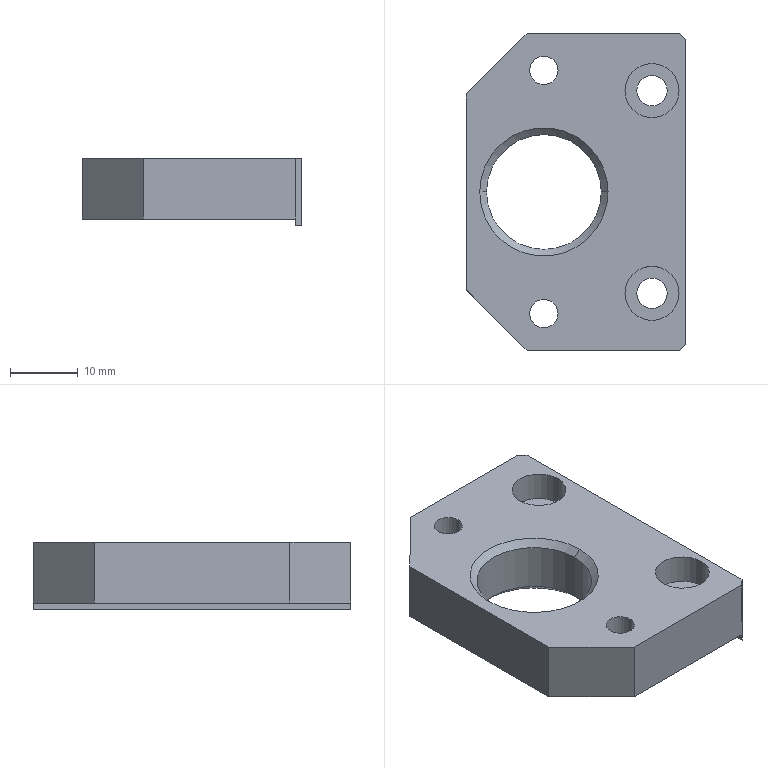Part | SolidWorks | features Chamfer 2, HoleWzd 2, ICE 2, Extrusion 1 | 1 solid | 32 faces | box 32.5 x 47 x 10 mm | volume 10119 mm3 | cylinder 14 | plane 14 | cone 4 | commonest cylinder face diameters 4.2 x4 4.5 x4 8 x4 17 x2
STEP:
#1=CARTESIAN_POINT('',(-13.25,0.,4.));
#2=VERTEX_POINT('',#1);
#3=CARTESIAN_POINT('',(3.75,0.,4.));
#4=VERTEX_POINT('',#3);
#5=CARTESIAN_POINT('',(-4.75,0.,4.));
#6=DIRECTION('',(0.,0.,1.));
#7=DIRECTION('',(-1.,0.,0.));
#8=AXIS2_PLACEMENT_3D('',#5,#6,#7);
#9=CIRCLE('',#8,8.5);
#10=EDGE_CURVE('',#2,#4,#9,.T.);
#11=ORIENTED_EDGE('',*,*,#10,.F.);
#12=CARTESIAN_POINT('',(-14.25,0.,5.));
#13=VERTEX_POINT('',#12);
#14=CARTESIAN_POINT('',(-13.25,0.,4.));
#15=DIRECTION('',(-0.7071,0.,0.7071));
#16=VECTOR('',#15,1000.);
#17=LINE('',#14,#16);
#18=EDGE_CURVE('',#2,#13,#17,.T.);
#19=ORIENTED_EDGE('',*,*,#18,.T.);
#20=CARTESIAN_POINT('',(4.75,0.,5.));
#21=VERTEX_POINT('',#20);
#22=CARTESIAN_POINT('',(-4.75,0.,5.));
#23=DIRECTION('',(0.,0.,-1.));
#24=DIRECTION('',(-1.,0.,0.));
#25=AXIS2_PLACEMENT_3D('',#22,#23,#24);
#26=CIRCLE('',#25,9.5);
#27=EDGE_CURVE('',#21,#13,#26,.T.);
#28=ORIENTED_EDGE('',*,*,#27,.F.);
#29=CARTESIAN_POINT('',(3.75,0.,4.));
#30=DIRECTION('',(0.7071,0.,0.7071));
#31=VECTOR('',#30,1000.);
#32=LINE('',#29,#31);
#33=EDGE_CURVE('',#4,#21,#32,.T.);
#34=ORIENTED_EDGE('',*,*,#33,.F.);
#35=EDGE_LOOP('',(#11,#19,#28,#34));
#36=FACE_OUTER_BOUND('',#35,.T.);
#37=CARTESIAN_POINT('',(-4.75,0.,4.));
#38=DIRECTION('',(0.,0.,1.));
#39=DIRECTION('',(1.,0.,0.));
#40=AXIS2_PLACEMENT_3D('',#37,#38,#39);
#41=CONICAL_SURFACE('',#40,8.5,0.7854);
#42=ADVANCED_FACE('',(#36),#41,.F.);
#43=CARTESIAN_POINT('',(3.75,0.,-3.));
#44=VERTEX_POINT('',#43);
#45=CARTESIAN_POINT('',(-13.25,0.,-3.));
#46=VERTEX_POINT('',#45);
#47=CARTESIAN_POINT('',(-4.75,0.,-3.));
#48=DIRECTION('',(0.,0.,-1.));
#49=DIRECTION('',(-1.,0.,0.));
#50=AXIS2_PLACEMENT_3D('',#47,#48,#49);
#51=CIRCLE('',#50,8.5);
#52=EDGE_CURVE('',#44,#46,#51,.T.);
#53=ORIENTED_EDGE('',*,*,#52,.F.);
#54=CARTESIAN_POINT('',(4.75,0.,-4.));
#55=VERTEX_POINT('',#54);
#56=CARTESIAN_POINT('',(3.75,0.,-3.));
#57=DIRECTION('',(0.7071,0.,-0.7071));
#58=VECTOR('',#57,1000.);
#59=LINE('',#56,#58);
#60=EDGE_CURVE('',#44,#55,#59,.T.);
#61=ORIENTED_EDGE('',*,*,#60,.T.);
#62=CARTESIAN_POINT('',(-14.25,0.,-4.));
#63=VERTEX_POINT('',#62);
#64=CARTESIAN_POINT('',(-4.75,0.,-4.));
#65=DIRECTION('',(0.,0.,1.));
#66=DIRECTION('',(-1.,0.,0.));
#67=AXIS2_PLACEMENT_3D('',#64,#65,#66);
#68=CIRCLE('',#67,9.5);
#69=EDGE_CURVE('',#63,#55,#68,.T.);
#70=ORIENTED_EDGE('',*,*,#69,.F.);
#71=CARTESIAN_POINT('',(-13.25,0.,-3.));
#72=DIRECTION('',(-0.7071,0.,-0.7071));
#73=VECTOR('',#72,1000.);
#74=LINE('',#71,#73);
#75=EDGE_CURVE('',#46,#63,#74,.T.);
#76=ORIENTED_EDGE('',*,*,#75,.F.);
#77=EDGE_LOOP('',(#53,#61,#70,#76));
#78=FACE_OUTER_BOUND('',#77,.T.);
#79=CARTESIAN_POINT('',(-4.75,0.,-3.));
#80=DIRECTION('',(0.,0.,-1.));
#81=DIRECTION('',(-1.,0.,0.));
#82=AXIS2_PLACEMENT_3D('',#79,#80,#81);
#83=CONICAL_SURFACE('',#82,8.5,0.7854);
#84=ADVANCED_FACE('',(#78),#83,.F.);
#85=ORIENTED_EDGE('',*,*,#52,.T.);
#86=CARTESIAN_POINT('',(-13.25,0.,-5.));
#87=DIRECTION('',(0.,0.,1.));
#88=VECTOR('',#87,1000.);
#89=LINE('',#86,#88);
#90=EDGE_CURVE('',#46,#2,#89,.T.);
#91=ORIENTED_EDGE('',*,*,#90,.T.);
#92=ORIENTED_EDGE('',*,*,#10,.T.);
#93=CARTESIAN_POINT('',(3.75,0.,-5.));
#94=DIRECTION('',(0.,0.,1.));
#95=VECTOR('',#94,1000.);
#96=LINE('',#93,#95);
#97=EDGE_CURVE('',#44,#4,#96,.T.);
#98=ORIENTED_EDGE('',*,*,#97,.F.);
#99=EDGE_LOOP('',(#85,#91,#92,#98));
#100=FACE_OUTER_BOUND('',#99,.T.);
#101=CARTESIAN_POINT('',(-4.75,0.,-5.));
#102=DIRECTION('',(0.,0.,1.));
#103=DIRECTION('',(1.,0.,0.));
#104=AXIS2_PLACEMENT_3D('',#101,#102,#103);
#105=CYLINDRICAL_SURFACE('',#104,8.5);
#106=ADVANCED_FACE('',(#100),#105,.F.);
#107=CARTESIAN_POINT('',(-2.65,18.,-4.));
#108=VERTEX_POINT('',#107);
#109=CARTESIAN_POINT('',(-6.85,18.,-4.));
#110=VERTEX_POINT('',#109);
#111=CARTESIAN_POINT('',(-4.75,18.,-4.));
#112=DIRECTION('',(0.,0.,-1.));
#113=DIRECTION('',(-1.,0.,0.));
#114=AXIS2_PLACEMENT_3D('',#111,#112,#113);
#115=CIRCLE('',#114,2.1);
#116=EDGE_CURVE('',#108,#110,#115,.T.);
#117=ORIENTED_EDGE('',*,*,#116,.T.);
#118=CARTESIAN_POINT('',(-6.85,18.,5.));
#119=VERTEX_POINT('',#118);
#120=CARTESIAN_POINT('',(-6.85,18.,5.));
#121=DIRECTION('',(0.,0.,1.));
#122=VECTOR('',#121,1000.);
#123=LINE('',#120,#122);
#124=EDGE_CURVE('',#110,#119,#123,.T.);
#125=ORIENTED_EDGE('',*,*,#124,.T.);
#126=CARTESIAN_POINT('',(-2.65,18.,5.));
#127=VERTEX_POINT('',#126);
#128=CARTESIAN_POINT('',(-4.75,18.,5.));
#129=DIRECTION('',(0.,0.,1.));
#130=DIRECTION('',(1.,0.,0.));
#131=AXIS2_PLACEMENT_3D('',#128,#129,#130);
#132=CIRCLE('',#131,2.1);
#133=EDGE_CURVE('',#119,#127,#132,.T.);
#134=ORIENTED_EDGE('',*,*,#133,.T.);
#135=CARTESIAN_POINT('',(-2.65,18.,5.));
#136=DIRECTION('',(0.,0.,1.));
#137=VECTOR('',#136,1000.);
#138=LINE('',#135,#137);
#139=EDGE_CURVE('',#108,#127,#138,.T.);
#140=ORIENTED_EDGE('',*,*,#139,.F.);
#141=EDGE_LOOP('',(#117,#125,#134,#140));
#142=FACE_OUTER_BOUND('',#141,.T.);
#143=CARTESIAN_POINT('',(-4.75,18.,5.));
#144=DIRECTION('',(0.,0.,1.));
#145=DIRECTION('',(1.,0.,0.));
#146=AXIS2_PLACEMENT_3D('',#143,#144,#145);
#147=CYLINDRICAL_SURFACE('',#146,2.1);
#148=ADVANCED_FACE('',(#142),#147,.F.);
#149=CARTESIAN_POINT('',(-2.65,-18.,-4.));
#150=VERTEX_POINT('',#149);
#151=CARTESIAN_POINT('',(-6.85,-18.,-4.));
#152=VERTEX_POINT('',#151);
#153=CARTESIAN_POINT('',(-4.75,-18.,-4.));
#154=DIRECTION('',(0.,0.,-1.));
#155=DIRECTION('',(-1.,0.,0.));
#156=AXIS2_PLACEMENT_3D('',#153,#154,#155);
#157=CIRCLE('',#156,2.1);
#158=EDGE_CURVE('',#150,#152,#157,.T.);
#159=ORIENTED_EDGE('',*,*,#158,.T.);
#160=CARTESIAN_POINT('',(-6.85,-18.,5.));
#161=VERTEX_POINT('',#160);
#162=CARTESIAN_POINT('',(-6.85,-18.,5.));
#163=DIRECTION('',(0.,0.,1.));
#164=VECTOR('',#163,1000.);
#165=LINE('',#162,#164);
#166=EDGE_CURVE('',#152,#161,#165,.T.);
#167=ORIENTED_EDGE('',*,*,#166,.T.);
#168=CARTESIAN_POINT('',(-2.65,-18.,5.));
#169=VERTEX_POINT('',#168);
#170=CARTESIAN_POINT('',(-4.75,-18.,5.));
#171=DIRECTION('',(0.,0.,1.));
#172=DIRECTION('',(1.,0.,0.));
#173=AXIS2_PLACEMENT_3D('',#170,#171,#172);
#174=CIRCLE('',#173,2.1);
#175=EDGE_CURVE('',#161,#169,#174,.T.);
#176=ORIENTED_EDGE('',*,*,#175,.T.);
#177=CARTESIAN_POINT('',(-2.65,-18.,5.));
#178=DIRECTION('',(0.,0.,1.));
#179=VECTOR('',#178,1000.);
#180=LINE('',#177,#179);
#181=EDGE_CURVE('',#150,#169,#180,.T.);
#182=ORIENTED_EDGE('',*,*,#181,.F.);
#183=EDGE_LOOP('',(#159,#167,#176,#182));
#184=FACE_OUTER_BOUND('',#183,.T.);
#185=CARTESIAN_POINT('',(-4.75,-18.,5.));
#186=DIRECTION('',(0.,0.,1.));
#187=DIRECTION('',(1.,0.,0.));
#188=AXIS2_PLACEMENT_3D('',#185,#186,#187);
#189=CYLINDRICAL_SURFACE('',#188,2.1);
#190=ADVANCED_FACE('',(#184),#189,.F.);
#191=CARTESIAN_POINT('',(7.25,15.,0.6));
#192=VERTEX_POINT('',#191);
#193=CARTESIAN_POINT('',(15.25,15.,0.6));
#194=VERTEX_POINT('',#193);
#195=CARTESIAN_POINT('',(11.25,15.,0.6));
#196=DIRECTION('',(0.,0.,1.));
#197=DIRECTION('',(1.,0.,0.));
#198=AXIS2_PLACEMENT_3D('',#195,#196,#197);
#199=CIRCLE('',#198,4.);
#200=EDGE_CURVE('',#192,#194,#199,.T.);
#201=ORIENTED_EDGE('',*,*,#200,.F.);
#202=CARTESIAN_POINT('',(7.25,15.,5.));
#203=VERTEX_POINT('',#202);
#204=CARTESIAN_POINT('',(7.25,15.,5.));
#205=DIRECTION('',(0.,0.,1.));
#206=VECTOR('',#205,1000.);
#207=LINE('',#204,#206);
#208=EDGE_CURVE('',#192,#203,#207,.T.);
#209=ORIENTED_EDGE('',*,*,#208,.T.);
#210=CARTESIAN_POINT('',(15.25,15.,5.));
#211=VERTEX_POINT('',#210);
#212=CARTESIAN_POINT('',(11.25,15.,5.));
#213=DIRECTION('',(0.,0.,1.));
#214=DIRECTION('',(1.,0.,0.));
#215=AXIS2_PLACEMENT_3D('',#212,#213,#214);
#216=CIRCLE('',#215,4.);
#217=EDGE_CURVE('',#203,#211,#216,.T.);
#218=ORIENTED_EDGE('',*,*,#217,.T.);
#219=CARTESIAN_POINT('',(15.25,15.,5.));
#220=DIRECTION('',(0.,0.,1.));
#221=VECTOR('',#220,1000.);
#222=LINE('',#219,#221);
#223=EDGE_CURVE('',#194,#211,#222,.T.);
#224=ORIENTED_EDGE('',*,*,#223,.F.);
#225=EDGE_LOOP('',(#201,#209,#218,#224));
#226=FACE_OUTER_BOUND('',#225,.T.);
#227=CARTESIAN_POINT('',(11.25,15.,5.));
#228=DIRECTION('',(0.,0.,1.));
#229=DIRECTION('',(1.,0.,0.));
#230=AXIS2_PLACEMENT_3D('',#227,#228,#229);
#231=CYLINDRICAL_SURFACE('',#230,4.);
#232=ADVANCED_FACE('',(#226),#231,.F.);
#233=CARTESIAN_POINT('',(7.25,-15.,0.6));
#234=VERTEX_POINT('',#233);
#235=CARTESIAN_POINT('',(15.25,-15.,0.6));
#236=VERTEX_POINT('',#235);
#237=CARTESIAN_POINT('',(11.25,-15.,0.6));
#238=DIRECTION('',(0.,0.,1.));
#239=DIRECTION('',(1.,0.,0.));
#240=AXIS2_PLACEMENT_3D('',#237,#238,#239);
#241=CIRCLE('',#240,4.);
#242=EDGE_CURVE('',#234,#236,#241,.T.);
#243=ORIENTED_EDGE('',*,*,#242,.F.);
#244=CARTESIAN_POINT('',(7.25,-15.,5.));
#245=VERTEX_POINT('',#244);
#246=CARTESIAN_POINT('',(7.25,-15.,5.));
#247=DIRECTION('',(0.,0.,1.));
#248=VECTOR('',#247,1000.);
#249=LINE('',#246,#248);
#250=EDGE_CURVE('',#234,#245,#249,.T.);
#251=ORIENTED_EDGE('',*,*,#250,.T.);
#252=CARTESIAN_POINT('',(15.25,-15.,5.));
#253=VERTEX_POINT('',#252);
#254=CARTESIAN_POINT('',(11.25,-15.,5.));
#255=DIRECTION('',(0.,0.,1.));
#256=DIRECTION('',(1.,0.,0.));
#257=AXIS2_PLACEMENT_3D('',#254,#255,#256);
#258=CIRCLE('',#257,4.);
#259=EDGE_CURVE('',#245,#253,#258,.T.);
#260=ORIENTED_EDGE('',*,*,#259,.T.);
#261=CARTESIAN_POINT('',(15.25,-15.,5.));
#262=DIRECTION('',(0.,0.,1.));
#263=VECTOR('',#262,1000.);
#264=LINE('',#261,#263);
#265=EDGE_CURVE('',#236,#253,#264,.T.);
#266=ORIENTED_EDGE('',*,*,#265,.F.);
#267=EDGE_LOOP('',(#243,#251,#260,#266));
#268=FACE_OUTER_BOUND('',#267,.T.);
#269=CARTESIAN_POINT('',(11.25,-15.,5.));
#270=DIRECTION('',(0.,0.,1.));
#271=DIRECTION('',(1.,0.,0.));
#272=AXIS2_PLACEMENT_3D('',#269,#270,#271);
#273=CYLINDRICAL_SURFACE('',#272,4.);
#274=ADVANCED_FACE('',(#268),#273,.F.);
#275=CARTESIAN_POINT('',(9.,15.,-4.));
#276=VERTEX_POINT('',#275);
#277=CARTESIAN_POINT('',(13.5,15.,-4.));
#278=VERTEX_POINT('',#277);
#279=CARTESIAN_POINT('',(11.25,15.,-4.));
#280=DIRECTION('',(0.,0.,1.));
#281=DIRECTION('',(-1.,0.,0.));
#282=AXIS2_PLACEMENT_3D('',#279,#280,#281);
#283=CIRCLE('',#282,2.25);
#284=EDGE_CURVE('',#276,#278,#283,.T.);
#285=ORIENTED_EDGE('',*,*,#284,.F.);
#286=CARTESIAN_POINT('',(9.,15.,0.6));
#287=VERTEX_POINT('',#286);
#288=CARTESIAN_POINT('',(9.,15.,5.));
#289=DIRECTION('',(0.,0.,1.));
#290=VECTOR('',#289,1000.);
#291=LINE('',#288,#290);
#292=EDGE_CURVE('',#276,#287,#291,.T.);
#293=ORIENTED_EDGE('',*,*,#292,.T.);
#294=CARTESIAN_POINT('',(13.5,15.,0.6));
#295=VERTEX_POINT('',#294);
#296=CARTESIAN_POINT('',(11.25,15.,0.6));
#297=DIRECTION('',(0.,0.,1.));
#298=DIRECTION('',(1.,0.,0.));
#299=AXIS2_PLACEMENT_3D('',#296,#297,#298);
#300=CIRCLE('',#299,2.25);
#301=EDGE_CURVE('',#287,#295,#300,.T.);
#302=ORIENTED_EDGE('',*,*,#301,.T.);
#303=CARTESIAN_POINT('',(13.5,15.,5.));
#304=DIRECTION('',(0.,0.,1.));
#305=VECTOR('',#304,1000.);
#306=LINE('',#303,#305);
#307=EDGE_CURVE('',#278,#295,#306,.T.);
#308=ORIENTED_EDGE('',*,*,#307,.F.);
#309=EDGE_LOOP('',(#285,#293,#302,#308));
#310=FACE_OUTER_BOUND('',#309,.T.);
#311=CARTESIAN_POINT('',(11.25,15.,5.));
#312=DIRECTION('',(0.,0.,1.));
#313=DIRECTION('',(1.,0.,0.));
#314=AXIS2_PLACEMENT_3D('',#311,#312,#313);
#315=CYLINDRICAL_SURFACE('',#314,2.25);
#316=ADVANCED_FACE('',(#310),#315,.F.);
#317=CARTESIAN_POINT('',(9.,-15.,-4.));
#318=VERTEX_POINT('',#317);
#319=CARTESIAN_POINT('',(13.5,-15.,-4.));
#320=VERTEX_POINT('',#319);
#321=CARTESIAN_POINT('',(11.25,-15.,-4.));
#322=DIRECTION('',(0.,0.,1.));
#323=DIRECTION('',(-1.,0.,0.));
#324=AXIS2_PLACEMENT_3D('',#321,#322,#323);
#325=CIRCLE('',#324,2.25);
#326=EDGE_CURVE('',#318,#320,#325,.T.);
#327=ORIENTED_EDGE('',*,*,#326,.F.);
#328=CARTESIAN_POINT('',(9.,-15.,0.6));
#329=VERTEX_POINT('',#328);
#330=CARTESIAN_POINT('',(9.,-15.,5.));
#331=DIRECTION('',(0.,0.,1.));
#332=VECTOR('',#331,1000.);
#333=LINE('',#330,#332);
#334=EDGE_CURVE('',#318,#329,#333,.T.);
#335=ORIENTED_EDGE('',*,*,#334,.T.);
#336=CARTESIAN_POINT('',(13.5,-15.,0.6));
#337=VERTEX_POINT('',#336);
#338=CARTESIAN_POINT('',(11.25,-15.,0.6));
#339=DIRECTION('',(0.,0.,1.));
#340=DIRECTION('',(1.,0.,0.));
#341=AXIS2_PLACEMENT_3D('',#338,#339,#340);
#342=CIRCLE('',#341,2.25);
#343=EDGE_CURVE('',#329,#337,#342,.T.);
#344=ORIENTED_EDGE('',*,*,#343,.T.);
#345=CARTESIAN_POINT('',(13.5,-15.,5.));
#346=DIRECTION('',(0.,0.,1.));
#347=VECTOR('',#346,1000.);
#348=LINE('',#345,#347);
#349=EDGE_CURVE('',#320,#337,#348,.T.);
#350=ORIENTED_EDGE('',*,*,#349,.F.);
#351=EDGE_LOOP('',(#327,#335,#344,#350));
#352=FACE_OUTER_BOUND('',#351,.T.);
#353=CARTESIAN_POINT('',(11.25,-15.,5.));
#354=DIRECTION('',(0.,0.,1.));
#355=DIRECTION('',(1.,0.,0.));
#356=AXIS2_PLACEMENT_3D('',#353,#354,#355);
#357=CYLINDRICAL_SURFACE('',#356,2.25);
#358=ADVANCED_FACE('',(#352),#357,.F.);
#359=CARTESIAN_POINT('',(-16.25,14.5,5.));
#360=VERTEX_POINT('',#359);
#361=CARTESIAN_POINT('',(-16.25,-14.5,5.));
#362=VERTEX_POINT('',#361);
#363=CARTESIAN_POINT('',(-16.25,-23.5,5.));
#364=DIRECTION('',(0.,-1.,0.));
#365=VECTOR('',#364,1000.);
#366=LINE('',#363,#365);
#367=EDGE_CURVE('',#360,#362,#366,.T.);
#368=ORIENTED_EDGE('',*,*,#367,.F.);
#369=CARTESIAN_POINT('',(-16.25,14.5,-4.));
#370=VERTEX_POINT('',#369);
#371=CARTESIAN_POINT('',(-16.25,14.5,5.));
#372=DIRECTION('',(0.,0.,-1.));
#373=VECTOR('',#372,1000.);
#374=LINE('',#371,#373);
#375=EDGE_CURVE('',#360,#370,#374,.T.);
#376=ORIENTED_EDGE('',*,*,#375,.T.);
#377=CARTESIAN_POINT('',(-16.25,-14.5,-4.));
#378=VERTEX_POINT('',#377);
#379=CARTESIAN_POINT('',(-16.25,-23.5,-4.));
#380=DIRECTION('',(0.,1.,0.));
#381=VECTOR('',#380,1000.);
#382=LINE('',#379,#381);
#383=EDGE_CURVE('',#378,#370,#382,.T.);
#384=ORIENTED_EDGE('',*,*,#383,.F.);
#385=CARTESIAN_POINT('',(-16.25,-14.5,5.));
#386=DIRECTION('',(0.,0.,1.));
#387=VECTOR('',#386,1000.);
#388=LINE('',#385,#387);
#389=EDGE_CURVE('',#378,#362,#388,.T.);
#390=ORIENTED_EDGE('',*,*,#389,.T.);
#391=EDGE_LOOP('',(#368,#376,#384,#390));
#392=FACE_OUTER_BOUND('',#391,.T.);
#393=CARTESIAN_POINT('',(-16.25,-23.5,5.));
#394=DIRECTION('',(1.,0.,0.));
#395=DIRECTION('',(0.,0.,-1.));
#396=AXIS2_PLACEMENT_3D('',#393,#394,#395);
#397=PLANE('',#396);
#398=ADVANCED_FACE('',(#392),#397,.F.);
#399=ORIENTED_EDGE('',*,*,#334,.F.);
#400=CARTESIAN_POINT('',(11.25,-15.,-4.));
#401=DIRECTION('',(0.,0.,1.));
#402=DIRECTION('',(-1.,0.,0.));
#403=AXIS2_PLACEMENT_3D('',#400,#401,#402);
#404=CIRCLE('',#403,2.25);
#405=EDGE_CURVE('',#320,#318,#404,.T.);
#406=ORIENTED_EDGE('',*,*,#405,.F.);
#407=ORIENTED_EDGE('',*,*,#349,.T.);
#408=CARTESIAN_POINT('',(11.25,-15.,0.6));
#409=DIRECTION('',(0.,0.,1.));
#410=DIRECTION('',(1.,0.,0.));
#411=AXIS2_PLACEMENT_3D('',#408,#409,#410);
#412=CIRCLE('',#411,2.25);
#413=EDGE_CURVE('',#337,#329,#412,.T.);
#414=ORIENTED_EDGE('',*,*,#413,.T.);
#415=EDGE_LOOP('',(#399,#406,#407,#414));
#416=FACE_OUTER_BOUND('',#415,.T.);
#417=CARTESIAN_POINT('',(11.25,-15.,5.));
#418=DIRECTION('',(0.,0.,1.));
#419=DIRECTION('',(1.,0.,0.));
#420=AXIS2_PLACEMENT_3D('',#417,#418,#419);
#421=CYLINDRICAL_SURFACE('',#420,2.25);
#422=ADVANCED_FACE('',(#416),#421,.F.);
#423=ORIENTED_EDGE('',*,*,#292,.F.);
#424=CARTESIAN_POINT('',(11.25,15.,-4.));
#425=DIRECTION('',(0.,0.,1.));
#426=DIRECTION('',(-1.,0.,0.));
#427=AXIS2_PLACEMENT_3D('',#424,#425,#426);
#428=CIRCLE('',#427,2.25);
#429=EDGE_CURVE('',#278,#276,#428,.T.);
#430=ORIENTED_EDGE('',*,*,#429,.F.);
#431=ORIENTED_EDGE('',*,*,#307,.T.);
#432=CARTESIAN_POINT('',(11.25,15.,0.6));
#433=DIRECTION('',(0.,0.,1.));
#434=DIRECTION('',(1.,0.,0.));
#435=AXIS2_PLACEMENT_3D('',#432,#433,#434);
#436=CIRCLE('',#435,2.25);
#437=EDGE_CURVE('',#295,#287,#436,.T.);
#438=ORIENTED_EDGE('',*,*,#437,.T.);
#439=EDGE_LOOP('',(#423,#430,#431,#438));
#440=FACE_OUTER_BOUND('',#439,.T.);
#441=CARTESIAN_POINT('',(11.25,15.,5.));
#442=DIRECTION('',(0.,0.,1.));
#443=DIRECTION('',(1.,0.,0.));
#444=AXIS2_PLACEMENT_3D('',#441,#442,#443);
#445=CYLINDRICAL_SURFACE('',#444,2.25);
#446=ADVANCED_FACE('',(#440),#445,.F.);
#447=CARTESIAN_POINT('',(16.25,-22.5,-5.));
#448=VERTEX_POINT('',#447);
#449=CARTESIAN_POINT('',(16.25,22.5,-5.));
#450=VERTEX_POINT('',#449);
#451=CARTESIAN_POINT('',(16.25,-23.5,-5.));
#452=DIRECTION('',(0.,1.,0.));
#453=VECTOR('',#452,1000.);
#454=LINE('',#451,#453);
#455=EDGE_CURVE('',#448,#450,#454,.T.);
#456=ORIENTED_EDGE('',*,*,#455,.T.);
#457=CARTESIAN_POINT('',(16.25,22.5,5.));
#458=VERTEX_POINT('',#457);
#459=CARTESIAN_POINT('',(16.25,22.5,5.));
#460=DIRECTION('',(0.,0.,1.));
#461=VECTOR('',#460,1000.);
#462=LINE('',#459,#461);
#463=EDGE_CURVE('',#450,#458,#462,.T.);
#464=ORIENTED_EDGE('',*,*,#463,.T.);
#465=CARTESIAN_POINT('',(16.25,-22.5,5.));
#466=VERTEX_POINT('',#465);
#467=CARTESIAN_POINT('',(16.25,-23.5,5.));
#468=DIRECTION('',(0.,1.,0.));
#469=VECTOR('',#468,1000.);
#470=LINE('',#467,#469);
#471=EDGE_CURVE('',#466,#458,#470,.T.);
#472=ORIENTED_EDGE('',*,*,#471,.F.);
#473=CARTESIAN_POINT('',(16.25,-22.5,5.));
#474=DIRECTION('',(0.,0.,-1.));
#475=VECTOR('',#474,1000.);
#476=LINE('',#473,#475);
#477=EDGE_CURVE('',#466,#448,#476,.T.);
#478=ORIENTED_EDGE('',*,*,#477,.T.);
#479=EDGE_LOOP('',(#456,#464,#472,#478));
#480=FACE_OUTER_BOUND('',#479,.T.);
#481=CARTESIAN_POINT('',(16.25,-23.5,5.));
#482=DIRECTION('',(-1.,0.,0.));
#483=DIRECTION('',(0.,0.,1.));
#484=AXIS2_PLACEMENT_3D('',#481,#482,#483);
#485=PLANE('',#484);
#486=ADVANCED_FACE('',(#480),#485,.F.);
#487=CARTESIAN_POINT('',(15.25,23.5,5.));
#488=VERTEX_POINT('',#487);
#489=CARTESIAN_POINT('',(-7.25,23.5,5.));
#490=VERTEX_POINT('',#489);
#491=CARTESIAN_POINT('',(-16.25,23.5,5.));
#492=DIRECTION('',(-1.,0.,0.));
#493=VECTOR('',#492,1000.);
#494=LINE('',#491,#493);
#495=EDGE_CURVE('',#488,#490,#494,.T.);
#496=ORIENTED_EDGE('',*,*,#495,.F.);
#497=CARTESIAN_POINT('',(15.25,23.5,-4.));
#498=VERTEX_POINT('',#497);
#499=CARTESIAN_POINT('',(15.25,23.5,5.));
#500=DIRECTION('',(0.,0.,-1.));
#501=VECTOR('',#500,1000.);
#502=LINE('',#499,#501);
#503=EDGE_CURVE('',#488,#498,#502,.T.);
#504=ORIENTED_EDGE('',*,*,#503,.T.);
#505=CARTESIAN_POINT('',(-7.25,23.5,-4.));
#506=VERTEX_POINT('',#505);
#507=CARTESIAN_POINT('',(-16.25,23.5,-4.));
#508=DIRECTION('',(1.,0.,0.));
#509=VECTOR('',#508,1000.);
#510=LINE('',#507,#509);
#511=EDGE_CURVE('',#506,#498,#510,.T.);
#512=ORIENTED_EDGE('',*,*,#511,.F.);
#513=CARTESIAN_POINT('',(-7.25,23.5,5.));
#514=DIRECTION('',(0.,0.,1.));
#515=VECTOR('',#514,1000.);
#516=LINE('',#513,#515);
#517=EDGE_CURVE('',#506,#490,#516,.T.);
#518=ORIENTED_EDGE('',*,*,#517,.T.);
#519=EDGE_LOOP('',(#496,#504,#512,#518));
#520=FACE_OUTER_BOUND('',#519,.T.);
#521=CARTESIAN_POINT('',(-16.25,23.5,5.));
#522=DIRECTION('',(0.,-1.,0.));
#523=DIRECTION('',(0.,0.,-1.));
#524=AXIS2_PLACEMENT_3D('',#521,#522,#523);
#525=PLANE('',#524);
#526=ADVANCED_FACE('',(#520),#525,.F.);
#527=CARTESIAN_POINT('',(15.25,-23.5,-4.));
#528=VERTEX_POINT('',#527);
#529=CARTESIAN_POINT('',(-7.25,-23.5,-4.));
#530=VERTEX_POINT('',#529);
#531=CARTESIAN_POINT('',(-16.25,-23.5,-4.));
#532=DIRECTION('',(-1.,0.,0.));
#533=VECTOR('',#532,1000.);
#534=LINE('',#531,#533);
#535=EDGE_CURVE('',#528,#530,#534,.T.);
#536=ORIENTED_EDGE('',*,*,#535,.F.);
#537=CARTESIAN_POINT('',(15.25,-23.5,5.));
#538=VERTEX_POINT('',#537);
#539=CARTESIAN_POINT('',(15.25,-23.5,5.));
#540=DIRECTION('',(0.,0.,1.));
#541=VECTOR('',#540,1000.);
#542=LINE('',#539,#541);
#543=EDGE_CURVE('',#528,#538,#542,.T.);
#544=ORIENTED_EDGE('',*,*,#543,.T.);
#545=CARTESIAN_POINT('',(-7.25,-23.5,5.));
#546=VERTEX_POINT('',#545);
#547=CARTESIAN_POINT('',(-16.25,-23.5,5.));
#548=DIRECTION('',(1.,0.,0.));
#549=VECTOR('',#548,1000.);
#550=LINE('',#547,#549);
#551=EDGE_CURVE('',#546,#538,#550,.T.);
#552=ORIENTED_EDGE('',*,*,#551,.F.);
#553=CARTESIAN_POINT('',(-7.25,-23.5,5.));
#554=DIRECTION('',(0.,0.,-1.));
#555=VECTOR('',#554,1000.);
#556=LINE('',#553,#555);
#557=EDGE_CURVE('',#546,#530,#556,.T.);
#558=ORIENTED_EDGE('',*,*,#557,.T.);
#559=EDGE_LOOP('',(#536,#544,#552,#558));
#560=FACE_OUTER_BOUND('',#559,.T.);
#561=CARTESIAN_POINT('',(-16.25,-23.5,5.));
#562=DIRECTION('',(0.,1.,0.));
#563=DIRECTION('',(0.,0.,1.));
#564=AXIS2_PLACEMENT_3D('',#561,#562,#563);
#565=PLANE('',#564);
#566=ADVANCED_FACE('',(#560),#565,.F.);
#567=ORIENTED_EDGE('',*,*,#27,.T.);
#568=CARTESIAN_POINT('',(-4.75,0.,5.));
#569=DIRECTION('',(0.,0.,-1.));
#570=DIRECTION('',(-1.,0.,0.));
#571=AXIS2_PLACEMENT_3D('',#568,#569,#570);
#572=CIRCLE('',#571,9.5);
#573=EDGE_CURVE('',#13,#21,#572,.T.);
#574=ORIENTED_EDGE('',*,*,#573,.T.);
#575=EDGE_LOOP('',(#567,#574));
#576=FACE_BOUND('',#575,.T.);
#577=CARTESIAN_POINT('',(-4.75,18.,5.));
#578=DIRECTION('',(0.,0.,1.));
#579=DIRECTION('',(1.,0.,0.));
#580=AXIS2_PLACEMENT_3D('',#577,#578,#579);
#581=CIRCLE('',#580,2.1);
#582=EDGE_CURVE('',#127,#119,#581,.T.);
#583=ORIENTED_EDGE('',*,*,#582,.F.);
#584=ORIENTED_EDGE('',*,*,#133,.F.);
#585=EDGE_LOOP('',(#583,#584));
#586=FACE_BOUND('',#585,.T.);
#587=CARTESIAN_POINT('',(-4.75,-18.,5.));
#588=DIRECTION('',(0.,0.,1.));
#589=DIRECTION('',(1.,0.,0.));
#590=AXIS2_PLACEMENT_3D('',#587,#588,#589);
#591=CIRCLE('',#590,2.1);
#592=EDGE_CURVE('',#169,#161,#591,.T.);
#593=ORIENTED_EDGE('',*,*,#592,.F.);
#594=ORIENTED_EDGE('',*,*,#175,.F.);
#595=EDGE_LOOP('',(#593,#594));
#596=FACE_BOUND('',#595,.T.);
#597=CARTESIAN_POINT('',(11.25,15.,5.));
#598=DIRECTION('',(0.,0.,1.));
#599=DIRECTION('',(1.,0.,0.));
#600=AXIS2_PLACEMENT_3D('',#597,#598,#599);
#601=CIRCLE('',#600,4.);
#602=EDGE_CURVE('',#211,#203,#601,.T.);
#603=ORIENTED_EDGE('',*,*,#602,.F.);
#604=ORIENTED_EDGE('',*,*,#217,.F.);
#605=EDGE_LOOP('',(#603,#604));
#606=FACE_BOUND('',#605,.T.);
#607=CARTESIAN_POINT('',(11.25,-15.,5.));
#608=DIRECTION('',(0.,0.,1.));
#609=DIRECTION('',(1.,0.,0.));
#610=AXIS2_PLACEMENT_3D('',#607,#608,#609);
#611=CIRCLE('',#610,4.);
#612=EDGE_CURVE('',#253,#245,#611,.T.);
#613=ORIENTED_EDGE('',*,*,#612,.F.);
#614=ORIENTED_EDGE('',*,*,#259,.F.);
#615=EDGE_LOOP('',(#613,#614));
#616=FACE_BOUND('',#615,.T.);
#617=ORIENTED_EDGE('',*,*,#471,.T.);
#618=CARTESIAN_POINT('',(15.25,23.5,5.));
#619=DIRECTION('',(-0.7071,0.7071,0.));
#620=VECTOR('',#619,1000.);
#621=LINE('',#618,#620);
#622=EDGE_CURVE('',#458,#488,#621,.T.);
#623=ORIENTED_EDGE('',*,*,#622,.T.);
#624=ORIENTED_EDGE('',*,*,#495,.T.);
#625=CARTESIAN_POINT('',(-16.25,14.5,5.));
#626=DIRECTION('',(-0.7071,-0.7071,0.));
#627=VECTOR('',#626,1000.);
#628=LINE('',#625,#627);
#629=EDGE_CURVE('',#490,#360,#628,.T.);
#630=ORIENTED_EDGE('',*,*,#629,.T.);
#631=ORIENTED_EDGE('',*,*,#367,.T.);
#632=CARTESIAN_POINT('',(-7.25,-23.5,5.));
#633=DIRECTION('',(0.7071,-0.7071,0.));
#634=VECTOR('',#633,1000.);
#635=LINE('',#632,#634);
#636=EDGE_CURVE('',#362,#546,#635,.T.);
#637=ORIENTED_EDGE('',*,*,#636,.T.);
#638=ORIENTED_EDGE('',*,*,#551,.T.);
#639=CARTESIAN_POINT('',(16.25,-22.5,5.));
#640=DIRECTION('',(0.7071,0.7071,0.));
#641=VECTOR('',#640,1000.);
#642=LINE('',#639,#641);
#643=EDGE_CURVE('',#538,#466,#642,.T.);
#644=ORIENTED_EDGE('',*,*,#643,.T.);
#645=EDGE_LOOP('',(#617,#623,#624,#630,#631,#637,#638,#644));
#646=FACE_OUTER_BOUND('',#645,.T.);
#647=CARTESIAN_POINT('',(0.,0.,5.));
#648=DIRECTION('',(0.,0.,-1.));
#649=DIRECTION('',(-1.,0.,0.));
#650=AXIS2_PLACEMENT_3D('',#647,#648,#649);
#651=PLANE('',#650);
#652=ADVANCED_FACE('',(#576,#586,#596,#606,#616,#646),#651,.F.);
#653=CARTESIAN_POINT('',(15.25,23.5,-5.));
#654=VERTEX_POINT('',#653);
#655=CARTESIAN_POINT('',(15.25,-23.5,-5.));
#656=VERTEX_POINT('',#655);
#657=CARTESIAN_POINT('',(15.25,-23.5,-5.));
#658=DIRECTION('',(0.,-1.,0.));
#659=VECTOR('',#658,1000.);
#660=LINE('',#657,#659);
#661=EDGE_CURVE('',#654,#656,#660,.T.);
#662=ORIENTED_EDGE('',*,*,#661,.F.);
#663=CARTESIAN_POINT('',(19.375,19.375,-5.));
#664=DIRECTION('',(0.7071,-0.7071,0.));
#665=VECTOR('',#664,1000.);
#666=LINE('',#663,#665);
#667=EDGE_CURVE('',#654,#450,#666,.T.);
#668=ORIENTED_EDGE('',*,*,#667,.T.);
#669=ORIENTED_EDGE('',*,*,#455,.F.);
#670=CARTESIAN_POINT('',(19.375,-19.375,-5.));
#671=DIRECTION('',(-0.7071,-0.7071,0.));
#672=VECTOR('',#671,1000.);
#673=LINE('',#670,#672);
#674=EDGE_CURVE('',#448,#656,#673,.T.);
#675=ORIENTED_EDGE('',*,*,#674,.T.);
#676=EDGE_LOOP('',(#662,#668,#669,#675));
#677=FACE_OUTER_BOUND('',#676,.T.);
#678=CARTESIAN_POINT('',(0.,0.,-5.));
#679=DIRECTION('',(0.,0.,-1.));
#680=DIRECTION('',(-1.,0.,0.));
#681=AXIS2_PLACEMENT_3D('',#678,#679,#680);
#682=PLANE('',#681);
#683=ADVANCED_FACE('',(#677),#682,.T.);
#684=ORIENTED_EDGE('',*,*,#413,.F.);
#685=ORIENTED_EDGE('',*,*,#343,.F.);
#686=EDGE_LOOP('',(#684,#685));
#687=FACE_BOUND('',#686,.T.);
#688=CARTESIAN_POINT('',(11.25,-15.,0.6));
#689=DIRECTION('',(0.,0.,1.));
#690=DIRECTION('',(1.,0.,0.));
#691=AXIS2_PLACEMENT_3D('',#688,#689,#690);
#692=CIRCLE('',#691,4.);
#693=EDGE_CURVE('',#236,#234,#692,.T.);
#694=ORIENTED_EDGE('',*,*,#693,.T.);
#695=ORIENTED_EDGE('',*,*,#242,.T.);
#696=EDGE_LOOP('',(#694,#695));
#697=FACE_OUTER_BOUND('',#696,.T.);
#698=CARTESIAN_POINT('',(13.5,-15.,0.6));
#699=DIRECTION('',(0.,0.,-1.));
#700=DIRECTION('',(-1.,0.,0.));
#701=AXIS2_PLACEMENT_3D('',#698,#699,#700);
#702=PLANE('',#701);
#703=ADVANCED_FACE('',(#687,#697),#702,.F.);
#704=ORIENTED_EDGE('',*,*,#250,.F.);
#705=ORIENTED_EDGE('',*,*,#693,.F.);
#706=ORIENTED_EDGE('',*,*,#265,.T.);
#707=ORIENTED_EDGE('',*,*,#612,.T.);
#708=EDGE_LOOP('',(#704,#705,#706,#707));
#709=FACE_OUTER_BOUND('',#708,.T.);
#710=CARTESIAN_POINT('',(11.25,-15.,5.));
#711=DIRECTION('',(0.,0.,1.));
#712=DIRECTION('',(1.,0.,0.));
#713=AXIS2_PLACEMENT_3D('',#710,#711,#712);
#714=CYLINDRICAL_SURFACE('',#713,4.);
#715=ADVANCED_FACE('',(#709),#714,.F.);
#716=ORIENTED_EDGE('',*,*,#437,.F.);
#717=ORIENTED_EDGE('',*,*,#301,.F.);
#718=EDGE_LOOP('',(#716,#717));
#719=FACE_BOUND('',#718,.T.);
#720=CARTESIAN_POINT('',(11.25,15.,0.6));
#721=DIRECTION('',(0.,0.,1.));
#722=DIRECTION('',(1.,0.,0.));
#723=AXIS2_PLACEMENT_3D('',#720,#721,#722);
#724=CIRCLE('',#723,4.);
#725=EDGE_CURVE('',#194,#192,#724,.T.);
#726=ORIENTED_EDGE('',*,*,#725,.T.);
#727=ORIENTED_EDGE('',*,*,#200,.T.);
#728=EDGE_LOOP('',(#726,#727));
#729=FACE_OUTER_BOUND('',#728,.T.);
#730=CARTESIAN_POINT('',(13.5,15.,0.6));
#731=DIRECTION('',(0.,0.,-1.));
#732=DIRECTION('',(-1.,0.,0.));
#733=AXIS2_PLACEMENT_3D('',#730,#731,#732);
#734=PLANE('',#733);
#735=ADVANCED_FACE('',(#719,#729),#734,.F.);
#736=ORIENTED_EDGE('',*,*,#208,.F.);
#737=ORIENTED_EDGE('',*,*,#725,.F.);
#738=ORIENTED_EDGE('',*,*,#223,.T.);
#739=ORIENTED_EDGE('',*,*,#602,.T.);
#740=EDGE_LOOP('',(#736,#737,#738,#739));
#741=FACE_OUTER_BOUND('',#740,.T.);
#742=CARTESIAN_POINT('',(11.25,15.,5.));
#743=DIRECTION('',(0.,0.,1.));
#744=DIRECTION('',(1.,0.,0.));
#745=AXIS2_PLACEMENT_3D('',#742,#743,#744);
#746=CYLINDRICAL_SURFACE('',#745,4.);
#747=ADVANCED_FACE('',(#741),#746,.F.);
#748=ORIENTED_EDGE('',*,*,#69,.T.);
#749=CARTESIAN_POINT('',(-4.75,0.,-4.));
#750=DIRECTION('',(0.,0.,1.));
#751=DIRECTION('',(-1.,0.,0.));
#752=AXIS2_PLACEMENT_3D('',#749,#750,#751);
#753=CIRCLE('',#752,9.5);
#754=EDGE_CURVE('',#55,#63,#753,.T.);
#755=ORIENTED_EDGE('',*,*,#754,.T.);
#756=EDGE_LOOP('',(#748,#755));
#757=FACE_BOUND('',#756,.T.);
#758=ORIENTED_EDGE('',*,*,#116,.F.);
#759=CARTESIAN_POINT('',(-4.75,18.,-4.));
#760=DIRECTION('',(0.,0.,-1.));
#761=DIRECTION('',(-1.,0.,0.));
#762=AXIS2_PLACEMENT_3D('',#759,#760,#761);
#763=CIRCLE('',#762,2.1);
#764=EDGE_CURVE('',#110,#108,#763,.T.);
#765=ORIENTED_EDGE('',*,*,#764,.F.);
#766=EDGE_LOOP('',(#758,#765));
#767=FACE_BOUND('',#766,.T.);
#768=ORIENTED_EDGE('',*,*,#158,.F.);
#769=CARTESIAN_POINT('',(-4.75,-18.,-4.));
#770=DIRECTION('',(0.,0.,-1.));
#771=DIRECTION('',(-1.,0.,0.));
#772=AXIS2_PLACEMENT_3D('',#769,#770,#771);
#773=CIRCLE('',#772,2.1);
#774=EDGE_CURVE('',#152,#150,#773,.T.);
#775=ORIENTED_EDGE('',*,*,#774,.F.);
#776=EDGE_LOOP('',(#768,#775));
#777=FACE_BOUND('',#776,.T.);
#778=ORIENTED_EDGE('',*,*,#429,.T.);
#779=ORIENTED_EDGE('',*,*,#284,.T.);
#780=EDGE_LOOP('',(#778,#779));
#781=FACE_BOUND('',#780,.T.);
#782=ORIENTED_EDGE('',*,*,#383,.T.);
#783=CARTESIAN_POINT('',(-15.375,15.375,-4.));
#784=DIRECTION('',(0.7071,0.7071,0.));
#785=VECTOR('',#784,1000.);
#786=LINE('',#783,#785);
#787=EDGE_CURVE('',#370,#506,#786,.T.);
#788=ORIENTED_EDGE('',*,*,#787,.T.);
#789=ORIENTED_EDGE('',*,*,#511,.T.);
#790=CARTESIAN_POINT('',(15.25,-23.5,-4.));
#791=DIRECTION('',(0.,-1.,0.));
#792=VECTOR('',#791,1000.);
#793=LINE('',#790,#792);
#794=EDGE_CURVE('',#498,#528,#793,.T.);
#795=ORIENTED_EDGE('',*,*,#794,.T.);
#796=ORIENTED_EDGE('',*,*,#535,.T.);
#797=CARTESIAN_POINT('',(-15.375,-15.375,-4.));
#798=DIRECTION('',(-0.7071,0.7071,0.));
#799=VECTOR('',#798,1000.);
#800=LINE('',#797,#799);
#801=EDGE_CURVE('',#530,#378,#800,.T.);
#802=ORIENTED_EDGE('',*,*,#801,.T.);
#803=EDGE_LOOP('',(#782,#788,#789,#795,#796,#802));
#804=FACE_OUTER_BOUND('',#803,.T.);
#805=ORIENTED_EDGE('',*,*,#405,.T.);
#806=ORIENTED_EDGE('',*,*,#326,.T.);
#807=EDGE_LOOP('',(#805,#806));
#808=FACE_BOUND('',#807,.T.);
#809=CARTESIAN_POINT('',(0.,0.,-4.));
#810=DIRECTION('',(0.,0.,-1.));
#811=DIRECTION('',(-1.,0.,0.));
#812=AXIS2_PLACEMENT_3D('',#809,#810,#811);
#813=PLANE('',#812);
#814=ADVANCED_FACE('',(#757,#767,#777,#781,#804,#808),#813,.T.);
#815=ORIENTED_EDGE('',*,*,#661,.T.);
#816=CARTESIAN_POINT('',(15.25,-23.5,-4.));
#817=DIRECTION('',(0.,0.,-1.));
#818=VECTOR('',#817,1000.);
#819=LINE('',#816,#818);
#820=EDGE_CURVE('',#528,#656,#819,.T.);
#821=ORIENTED_EDGE('',*,*,#820,.F.);
#822=ORIENTED_EDGE('',*,*,#794,.F.);
#823=CARTESIAN_POINT('',(15.25,23.5,-4.));
#824=DIRECTION('',(0.,0.,-1.));
#825=VECTOR('',#824,1000.);
#826=LINE('',#823,#825);
#827=EDGE_CURVE('',#498,#654,#826,.T.);
#828=ORIENTED_EDGE('',*,*,#827,.T.);
#829=EDGE_LOOP('',(#815,#821,#822,#828));
#830=FACE_OUTER_BOUND('',#829,.T.);
#831=CARTESIAN_POINT('',(15.25,-23.5,-4.));
#832=DIRECTION('',(1.,0.,0.));
#833=DIRECTION('',(0.,0.,-1.));
#834=AXIS2_PLACEMENT_3D('',#831,#832,#833);
#835=PLANE('',#834);
#836=ADVANCED_FACE('',(#830),#835,.F.);
#837=ORIENTED_EDGE('',*,*,#166,.F.);
#838=ORIENTED_EDGE('',*,*,#774,.T.);
#839=ORIENTED_EDGE('',*,*,#181,.T.);
#840=ORIENTED_EDGE('',*,*,#592,.T.);
#841=EDGE_LOOP('',(#837,#838,#839,#840));
#842=FACE_OUTER_BOUND('',#841,.T.);
#843=CARTESIAN_POINT('',(-4.75,-18.,5.));
#844=DIRECTION('',(0.,0.,1.));
#845=DIRECTION('',(1.,0.,0.));
#846=AXIS2_PLACEMENT_3D('',#843,#844,#845);
#847=CYLINDRICAL_SURFACE('',#846,2.1);
#848=ADVANCED_FACE('',(#842),#847,.F.);
#849=ORIENTED_EDGE('',*,*,#124,.F.);
#850=ORIENTED_EDGE('',*,*,#764,.T.);
#851=ORIENTED_EDGE('',*,*,#139,.T.);
#852=ORIENTED_EDGE('',*,*,#582,.T.);
#853=EDGE_LOOP('',(#849,#850,#851,#852));
#854=FACE_OUTER_BOUND('',#853,.T.);
#855=CARTESIAN_POINT('',(-4.75,18.,5.));
#856=DIRECTION('',(0.,0.,1.));
#857=DIRECTION('',(1.,0.,0.));
#858=AXIS2_PLACEMENT_3D('',#855,#856,#857);
#859=CYLINDRICAL_SURFACE('',#858,2.1);
#860=ADVANCED_FACE('',(#854),#859,.F.);
#861=ORIENTED_EDGE('',*,*,#90,.F.);
#862=CARTESIAN_POINT('',(-4.75,0.,-3.));
#863=DIRECTION('',(0.,0.,-1.));
#864=DIRECTION('',(-1.,0.,0.));
#865=AXIS2_PLACEMENT_3D('',#862,#863,#864);
#866=CIRCLE('',#865,8.5);
#867=EDGE_CURVE('',#46,#44,#866,.T.);
#868=ORIENTED_EDGE('',*,*,#867,.T.);
#869=ORIENTED_EDGE('',*,*,#97,.T.);
#870=CARTESIAN_POINT('',(-4.75,0.,4.));
#871=DIRECTION('',(0.,0.,1.));
#872=DIRECTION('',(-1.,0.,0.));
#873=AXIS2_PLACEMENT_3D('',#870,#871,#872);
#874=CIRCLE('',#873,8.5);
#875=EDGE_CURVE('',#4,#2,#874,.T.);
#876=ORIENTED_EDGE('',*,*,#875,.T.);
#877=EDGE_LOOP('',(#861,#868,#869,#876));
#878=FACE_OUTER_BOUND('',#877,.T.);
#879=CARTESIAN_POINT('',(-4.75,0.,-5.));
#880=DIRECTION('',(0.,0.,1.));
#881=DIRECTION('',(1.,0.,0.));
#882=AXIS2_PLACEMENT_3D('',#879,#880,#881);
#883=CYLINDRICAL_SURFACE('',#882,8.5);
#884=ADVANCED_FACE('',(#878),#883,.F.);
#885=ORIENTED_EDGE('',*,*,#629,.F.);
#886=ORIENTED_EDGE('',*,*,#517,.F.);
#887=ORIENTED_EDGE('',*,*,#787,.F.);
#888=ORIENTED_EDGE('',*,*,#375,.F.);
#889=EDGE_LOOP('',(#885,#886,#887,#888));
#890=FACE_OUTER_BOUND('',#889,.T.);
#891=CARTESIAN_POINT('',(-16.25,14.5,5.));
#892=DIRECTION('',(0.7071,-0.7071,0.));
#893=DIRECTION('',(0.,0.,-1.));
#894=AXIS2_PLACEMENT_3D('',#891,#892,#893);
#895=PLANE('',#894);
#896=ADVANCED_FACE('',(#890),#895,.F.);
#897=ORIENTED_EDGE('',*,*,#636,.F.);
#898=ORIENTED_EDGE('',*,*,#389,.F.);
#899=ORIENTED_EDGE('',*,*,#801,.F.);
#900=ORIENTED_EDGE('',*,*,#557,.F.);
#901=EDGE_LOOP('',(#897,#898,#899,#900));
#902=FACE_OUTER_BOUND('',#901,.T.);
#903=CARTESIAN_POINT('',(-7.25,-23.5,5.));
#904=DIRECTION('',(0.7071,0.7071,0.));
#905=DIRECTION('',(0.,0.,-1.));
#906=AXIS2_PLACEMENT_3D('',#903,#904,#905);
#907=PLANE('',#906);
#908=ADVANCED_FACE('',(#902),#907,.F.);
#909=ORIENTED_EDGE('',*,*,#60,.F.);
#910=ORIENTED_EDGE('',*,*,#867,.F.);
#911=ORIENTED_EDGE('',*,*,#75,.T.);
#912=ORIENTED_EDGE('',*,*,#754,.F.);
#913=EDGE_LOOP('',(#909,#910,#911,#912));
#914=FACE_OUTER_BOUND('',#913,.T.);
#915=CARTESIAN_POINT('',(-4.75,0.,-3.));
#916=DIRECTION('',(0.,0.,-1.));
#917=DIRECTION('',(-1.,0.,0.));
#918=AXIS2_PLACEMENT_3D('',#915,#916,#917);
#919=CONICAL_SURFACE('',#918,8.5,0.7854);
#920=ADVANCED_FACE('',(#914),#919,.F.);
#921=ORIENTED_EDGE('',*,*,#18,.F.);
#922=ORIENTED_EDGE('',*,*,#875,.F.);
#923=ORIENTED_EDGE('',*,*,#33,.T.);
#924=ORIENTED_EDGE('',*,*,#573,.F.);
#925=EDGE_LOOP('',(#921,#922,#923,#924));
#926=FACE_OUTER_BOUND('',#925,.T.);
#927=CARTESIAN_POINT('',(-4.75,0.,4.));
#928=DIRECTION('',(0.,0.,1.));
#929=DIRECTION('',(1.,0.,0.));
#930=AXIS2_PLACEMENT_3D('',#927,#928,#929);
#931=CONICAL_SURFACE('',#930,8.5,0.7854);
#932=ADVANCED_FACE('',(#926),#931,.F.);
#933=ORIENTED_EDGE('',*,*,#622,.F.);
#934=ORIENTED_EDGE('',*,*,#463,.F.);
#935=ORIENTED_EDGE('',*,*,#667,.F.);
#936=ORIENTED_EDGE('',*,*,#827,.F.);
#937=ORIENTED_EDGE('',*,*,#503,.F.);
#938=EDGE_LOOP('',(#933,#934,#935,#936,#937));
#939=FACE_OUTER_BOUND('',#938,.T.);
#940=CARTESIAN_POINT('',(15.25,23.5,5.));
#941=DIRECTION('',(-0.7071,-0.7071,0.));
#942=DIRECTION('',(0.,0.,-1.));
#943=AXIS2_PLACEMENT_3D('',#940,#941,#942);
#944=PLANE('',#943);
#945=ADVANCED_FACE('',(#939),#944,.F.);
#946=ORIENTED_EDGE('',*,*,#543,.F.);
#947=ORIENTED_EDGE('',*,*,#820,.T.);
#948=ORIENTED_EDGE('',*,*,#674,.F.);
#949=ORIENTED_EDGE('',*,*,#477,.F.);
#950=ORIENTED_EDGE('',*,*,#643,.F.);
#951=EDGE_LOOP('',(#946,#947,#948,#949,#950));
#952=FACE_OUTER_BOUND('',#951,.T.);
#953=CARTESIAN_POINT('',(16.25,-22.5,5.));
#954=DIRECTION('',(-0.7071,0.7071,0.));
#955=DIRECTION('',(0.,0.,-1.));
#956=AXIS2_PLACEMENT_3D('',#953,#954,#955);
#957=PLANE('',#956);
#958=ADVANCED_FACE('',(#952),#957,.F.);
#959=CLOSED_SHELL('',(#42,#84,#106,#148,#190,#232,#274,#316,#358,#398,#422,#446,#486,#526,#566,#652,#683,#703,#715,#735,#747,#814,#836,#848,#860,#884,#896,#908,#920,#932,#945,#958));
#960=MANIFOLD_SOLID_BREP('',#959);
#961=CARTESIAN_POINT('',(0.,0.,0.));
#962=DIRECTION('',(0.,0.,1.));
#963=DIRECTION('',(1.,0.,0.));
#964=AXIS2_PLACEMENT_3D('',#961,#962,#963);
#965=(LENGTH_UNIT()NAMED_UNIT(*)SI_UNIT(.MILLI.,.METRE.));
#966=UNCERTAINTY_MEASURE_WITH_UNIT(LENGTH_MEASURE(0.00001),#965,'','');
#967=(NAMED_UNIT(*)PLANE_ANGLE_UNIT()SI_UNIT($,.RADIAN.));
#968=(NAMED_UNIT(*)SI_UNIT($,.STERADIAN.)SOLID_ANGLE_UNIT());
#969=(GEOMETRIC_REPRESENTATION_CONTEXT(3)GLOBAL_UNCERTAINTY_ASSIGNED_CONTEXT((#966))GLOBAL_UNIT_ASSIGNED_CONTEXT((#965,#967,#968))REPRESENTATION_CONTEXT('',''));
#970=ADVANCED_BREP_SHAPE_REPRESENTATION('',(#960,#964),#969);